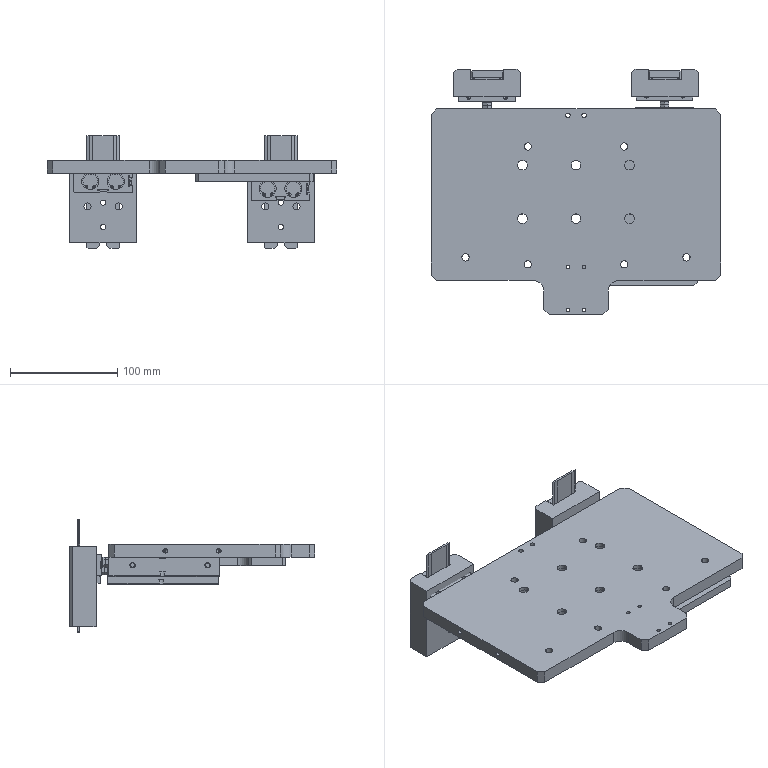Part | SolidWorks | features ReferencePattern 4, MirrorCompFeat 2 | 12 solids | 846 faces | box 270 x 229 x 105 mm | volume 1017603 mm3 | cylinder 401 | plane 331 | cone 114 | commonest cylinder face diameters 0.4 x60 1.52 x32 8 x32 3.5 x24 16 x24 9 x20